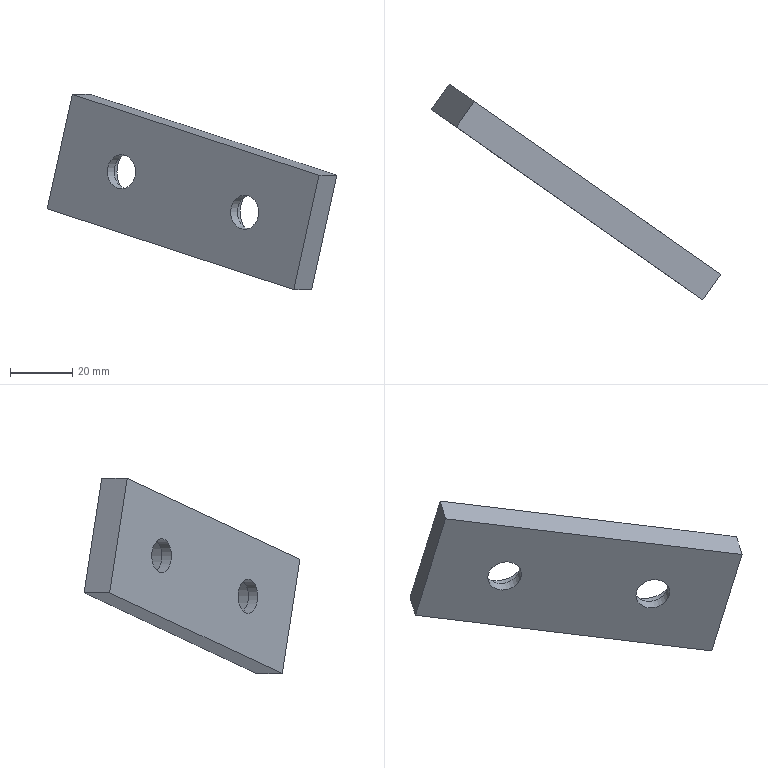Part | NX | features solid 2 | 1 solid | 12 faces | box 92.916 x 69.236 x 62.587 mm | volume 34266 mm3 | plane 8 | cylinder 4 | commonest cylinder face diameters 11 x2 17.5 x2
STEP:
#1=CARTESIAN_POINT('',(-114.685,856.129,30.673));
#2=VERTEX_POINT('',#1);
#3=CARTESIAN_POINT('',(-35.561,800.726,4.791));
#4=VERTEX_POINT('',#3);
#5=CARTESIAN_POINT('',(-109.761,852.681,29.063));
#6=DIRECTION('',(0.7912,-0.554,-0.2588));
#7=VECTOR('',#6,1000.);
#8=LINE('',#5,#7);
#9=EDGE_CURVE('',#2,#4,#8,.T.);
#10=ORIENTED_EDGE('',*,*,#9,.T.);
#11=CARTESIAN_POINT('',(-29.825,808.918,4.791));
#12=VERTEX_POINT('',#11);
#13=CARTESIAN_POINT('',(-29.825,808.918,4.791));
#14=DIRECTION('',(-0.5736,-0.8192,0.));
#15=VECTOR('',#14,1000.);
#16=LINE('',#13,#15);
#17=EDGE_CURVE('',#12,#4,#16,.T.);
#18=ORIENTED_EDGE('',*,*,#17,.F.);
#19=CARTESIAN_POINT('',(-108.949,864.321,30.673));
#20=VERTEX_POINT('',#19);
#21=CARTESIAN_POINT('',(-104.025,860.873,29.063));
#22=DIRECTION('',(0.7912,-0.554,-0.2588));
#23=VECTOR('',#22,1000.);
#24=LINE('',#21,#23);
#25=EDGE_CURVE('',#20,#12,#24,.T.);
#26=ORIENTED_EDGE('',*,*,#25,.F.);
#27=CARTESIAN_POINT('',(-108.949,864.321,30.673));
#28=DIRECTION('',(-0.5736,-0.8192,0.));
#29=VECTOR('',#28,1000.);
#30=LINE('',#27,#29);
#31=EDGE_CURVE('',#20,#2,#30,.T.);
#32=ORIENTED_EDGE('',*,*,#31,.T.);
#33=EDGE_LOOP('',(#10,#18,#26,#32));
#34=FACE_BOUND('',#33,.T.);
#35=CARTESIAN_POINT('',(-104.025,860.873,29.063));
#36=DIRECTION('',(0.212,-0.1485,0.9659));
#37=DIRECTION('',(-0.9676,-0.1706,0.1862));
#38=AXIS2_PLACEMENT_3D('',#35,#36,#37);
#39=PLANE('',#38);
#40=ADVANCED_FACE('',(#34),#39,.T.);
#41=CARTESIAN_POINT('',(-122.741,861.77,-6.032));
#42=VERTEX_POINT('',#41);
#43=CARTESIAN_POINT('',(-133.766,869.49,-56.26));
#44=DIRECTION('',(0.212,-0.1485,0.9659));
#45=VECTOR('',#44,1000.);
#46=LINE('',#43,#45);
#47=EDGE_CURVE('',#42,#2,#46,.T.);
#48=ORIENTED_EDGE('',*,*,#47,.T.);
#49=ORIENTED_EDGE('',*,*,#31,.F.);
#50=CARTESIAN_POINT('',(-117.005,869.962,-6.032));
#51=VERTEX_POINT('',#50);
#52=CARTESIAN_POINT('',(-128.03,877.681,-56.26));
#53=DIRECTION('',(0.212,-0.1485,0.9659));
#54=VECTOR('',#53,1000.);
#55=LINE('',#52,#54);
#56=EDGE_CURVE('',#51,#20,#55,.T.);
#57=ORIENTED_EDGE('',*,*,#56,.F.);
#58=CARTESIAN_POINT('',(-117.005,869.962,-6.032));
#59=DIRECTION('',(-0.5736,-0.8192,0.));
#60=VECTOR('',#59,1000.);
#61=LINE('',#58,#60);
#62=EDGE_CURVE('',#51,#42,#61,.T.);
#63=ORIENTED_EDGE('',*,*,#62,.T.);
#64=EDGE_LOOP('',(#48,#49,#57,#63));
#65=FACE_BOUND('',#64,.T.);
#66=CARTESIAN_POINT('',(-128.03,877.681,-56.26));
#67=DIRECTION('',(-0.7912,0.554,0.2588));
#68=DIRECTION('',(0.5736,0.8192,0.));
#69=AXIS2_PLACEMENT_3D('',#66,#67,#68);
#70=PLANE('',#69);
#71=ADVANCED_FACE('',(#65),#70,.T.);
#72=CARTESIAN_POINT('',(-43.617,806.367,-31.914));
#73=VERTEX_POINT('',#72);
#74=CARTESIAN_POINT('',(-117.817,858.323,-7.643));
#75=DIRECTION('',(0.7912,-0.554,-0.2588));
#76=VECTOR('',#75,1000.);
#77=LINE('',#74,#76);
#78=EDGE_CURVE('',#42,#73,#77,.T.);
#79=ORIENTED_EDGE('',*,*,#78,.F.);
#80=ORIENTED_EDGE('',*,*,#62,.F.);
#81=CARTESIAN_POINT('',(-37.881,814.559,-31.914));
#82=VERTEX_POINT('',#81);
#83=CARTESIAN_POINT('',(-112.081,866.514,-7.643));
#84=DIRECTION('',(0.7912,-0.554,-0.2588));
#85=VECTOR('',#84,1000.);
#86=LINE('',#83,#85);
#87=EDGE_CURVE('',#51,#82,#86,.T.);
#88=ORIENTED_EDGE('',*,*,#87,.T.);
#89=CARTESIAN_POINT('',(-37.881,814.559,-31.914));
#90=DIRECTION('',(-0.5736,-0.8192,0.));
#91=VECTOR('',#90,1000.);
#92=LINE('',#89,#91);
#93=EDGE_CURVE('',#82,#73,#92,.T.);
#94=ORIENTED_EDGE('',*,*,#93,.T.);
#95=EDGE_LOOP('',(#79,#80,#88,#94));
#96=FACE_BOUND('',#95,.T.);
#97=CARTESIAN_POINT('',(-112.081,866.514,-7.643));
#98=DIRECTION('',(0.212,-0.1485,0.9659));
#99=DIRECTION('',(-0.9676,-0.1706,0.1862));
#100=AXIS2_PLACEMENT_3D('',#97,#98,#99);
#101=PLANE('',#100);
#102=ADVANCED_FACE('',(#96),#101,.F.);
#103=CARTESIAN_POINT('',(-54.642,814.087,-82.142));
#104=DIRECTION('',(0.212,-0.1485,0.9659));
#105=VECTOR('',#104,1000.);
#106=LINE('',#103,#105);
#107=EDGE_CURVE('',#73,#4,#106,.T.);
#108=ORIENTED_EDGE('',*,*,#107,.F.);
#109=ORIENTED_EDGE('',*,*,#93,.F.);
#110=CARTESIAN_POINT('',(-48.906,822.278,-82.142));
#111=DIRECTION('',(0.212,-0.1485,0.9659));
#112=VECTOR('',#111,1000.);
#113=LINE('',#110,#112);
#114=EDGE_CURVE('',#82,#12,#113,.T.);
#115=ORIENTED_EDGE('',*,*,#114,.T.);
#116=ORIENTED_EDGE('',*,*,#17,.T.);
#117=EDGE_LOOP('',(#108,#109,#115,#116));
#118=FACE_BOUND('',#117,.T.);
#119=CARTESIAN_POINT('',(-48.906,822.278,-82.142));
#120=DIRECTION('',(-0.7912,0.554,0.2588));
#121=DIRECTION('',(0.5736,0.8192,0.));
#122=AXIS2_PLACEMENT_3D('',#119,#120,#121);
#123=PLANE('',#122);
#124=ADVANCED_FACE('',(#118),#123,.F.);
#125=CARTESIAN_POINT('',(-86.028,848.272,5.85));
#126=VERTEX_POINT('',#125);
#127=CARTESIAN_POINT('',(-93.196,853.291,5.85));
#128=DIRECTION('',(-0.5736,-0.8192,0.));
#129=DIRECTION('',(0.8192,-0.5736,0.));
#130=AXIS2_PLACEMENT_3D('',#127,#128,#129);
#131=CIRCLE('',#130,8.75);
#132=EDGE_CURVE('',#126,#126,#131,.T.);
#133=ORIENTED_EDGE('',*,*,#132,.T.);
#134=EDGE_LOOP('',(#133));
#135=FACE_BOUND('',#134,.T.);
#136=CARTESIAN_POINT('',(-46.466,820.57,-7.091));
#137=VERTEX_POINT('',#136);
#138=CARTESIAN_POINT('',(-53.634,825.589,-7.091));
#139=DIRECTION('',(-0.5736,-0.8192,0.));
#140=DIRECTION('',(0.8192,-0.5736,0.));
#141=AXIS2_PLACEMENT_3D('',#138,#139,#140);
#142=CIRCLE('',#141,8.75);
#143=EDGE_CURVE('',#137,#137,#142,.T.);
#144=ORIENTED_EDGE('',*,*,#143,.T.);
#145=EDGE_LOOP('',(#144));
#146=FACE_BOUND('',#145,.T.);
#147=ORIENTED_EDGE('',*,*,#25,.T.);
#148=ORIENTED_EDGE('',*,*,#114,.F.);
#149=ORIENTED_EDGE('',*,*,#87,.F.);
#150=ORIENTED_EDGE('',*,*,#56,.T.);
#151=EDGE_LOOP('',(#147,#148,#149,#150));
#152=FACE_BOUND('',#151,.T.);
#153=CARTESIAN_POINT('',(-123.106,874.234,-57.871));
#154=DIRECTION('',(0.5736,0.8192,0.));
#155=DIRECTION('',(0.8192,-0.5736,0.));
#156=AXIS2_PLACEMENT_3D('',#153,#154,#155);
#157=PLANE('',#156);
#158=ADVANCED_FACE('',(#135,#146,#152),#157,.T.);
#159=CARTESIAN_POINT('',(-103.437,848.254,5.85));
#160=VERTEX_POINT('',#159);
#161=CARTESIAN_POINT('',(-98.932,845.099,5.85));
#162=DIRECTION('',(0.5736,0.8192,0.));
#163=DIRECTION('',(-0.8192,0.5736,0.));
#164=AXIS2_PLACEMENT_3D('',#161,#162,#163);
#165=CIRCLE('',#164,5.5);
#166=EDGE_CURVE('',#160,#160,#165,.T.);
#167=ORIENTED_EDGE('',*,*,#166,.T.);
#168=EDGE_LOOP('',(#167));
#169=FACE_BOUND('',#168,.T.);
#170=CARTESIAN_POINT('',(-63.875,820.552,-7.091));
#171=VERTEX_POINT('',#170);
#172=CARTESIAN_POINT('',(-59.37,817.397,-7.091));
#173=DIRECTION('',(0.5736,0.8192,0.));
#174=DIRECTION('',(-0.8192,0.5736,0.));
#175=AXIS2_PLACEMENT_3D('',#172,#173,#174);
#176=CIRCLE('',#175,5.5);
#177=EDGE_CURVE('',#171,#171,#176,.T.);
#178=ORIENTED_EDGE('',*,*,#177,.T.);
#179=EDGE_LOOP('',(#178));
#180=FACE_BOUND('',#179,.T.);
#181=ORIENTED_EDGE('',*,*,#9,.F.);
#182=ORIENTED_EDGE('',*,*,#47,.F.);
#183=ORIENTED_EDGE('',*,*,#78,.T.);
#184=ORIENTED_EDGE('',*,*,#107,.T.);
#185=EDGE_LOOP('',(#181,#182,#183,#184));
#186=FACE_BOUND('',#185,.T.);
#187=CARTESIAN_POINT('',(-128.842,866.042,-57.871));
#188=DIRECTION('',(0.5736,0.8192,0.));
#189=DIRECTION('',(0.8192,-0.5736,0.));
#190=AXIS2_PLACEMENT_3D('',#187,#188,#189);
#191=PLANE('',#190);
#192=ADVANCED_FACE('',(#169,#180,#186),#191,.F.);
#193=CARTESIAN_POINT('',(-52.742,817.274,-7.091));
#194=VERTEX_POINT('',#193);
#195=CARTESIAN_POINT('',(-57.248,820.428,-7.091));
#196=DIRECTION('',(-0.5736,-0.8192,0.));
#197=DIRECTION('',(0.8192,-0.5736,0.));
#198=AXIS2_PLACEMENT_3D('',#195,#196,#197);
#199=CIRCLE('',#198,5.5);
#200=EDGE_CURVE('',#194,#194,#199,.T.);
#201=ORIENTED_EDGE('',*,*,#200,.F.);
#202=EDGE_LOOP('',(#201));
#203=FACE_BOUND('',#202,.T.);
#204=ORIENTED_EDGE('',*,*,#177,.F.);
#205=EDGE_LOOP('',(#204));
#206=FACE_BOUND('',#205,.T.);
#207=CARTESIAN_POINT('',(-82.313,784.631,-7.091));
#208=DIRECTION('',(-0.5736,-0.8192,0.));
#209=DIRECTION('',(0.8192,-0.5736,0.));
#210=AXIS2_PLACEMENT_3D('',#207,#208,#209);
#211=CYLINDRICAL_SURFACE('',#210,5.5);
#212=ADVANCED_FACE('',(#203,#206),#211,.F.);
#213=ORIENTED_EDGE('',*,*,#200,.T.);
#214=EDGE_LOOP('',(#213));
#215=FACE_BOUND('',#214,.T.);
#216=CARTESIAN_POINT('',(-50.08,815.409,-7.091));
#217=VERTEX_POINT('',#216);
#218=CARTESIAN_POINT('',(-57.248,820.428,-7.091));
#219=DIRECTION('',(-0.5736,-0.8192,0.));
#220=DIRECTION('',(0.8192,-0.5736,0.));
#221=AXIS2_PLACEMENT_3D('',#218,#219,#220);
#222=CIRCLE('',#221,8.75);
#223=EDGE_CURVE('',#217,#217,#222,.T.);
#224=ORIENTED_EDGE('',*,*,#223,.F.);
#225=EDGE_LOOP('',(#224));
#226=FACE_BOUND('',#225,.T.);
#227=CARTESIAN_POINT('',(-56.187,819.686,-2.261));
#228=DIRECTION('',(-0.5736,-0.8192,0.));
#229=DIRECTION('',(0.8192,-0.5736,0.));
#230=AXIS2_PLACEMENT_3D('',#227,#228,#229);
#231=PLANE('',#230);
#232=ADVANCED_FACE('',(#215,#226),#231,.F.);
#233=ORIENTED_EDGE('',*,*,#223,.T.);
#234=EDGE_LOOP('',(#233));
#235=FACE_BOUND('',#234,.T.);
#236=ORIENTED_EDGE('',*,*,#143,.F.);
#237=EDGE_LOOP('',(#236));
#238=FACE_BOUND('',#237,.T.);
#239=CARTESIAN_POINT('',(-53.634,825.589,-7.091));
#240=DIRECTION('',(-0.5736,-0.8192,0.));
#241=DIRECTION('',(0.8192,-0.5736,0.));
#242=AXIS2_PLACEMENT_3D('',#239,#240,#241);
#243=CYLINDRICAL_SURFACE('',#242,8.75);
#244=ADVANCED_FACE('',(#235,#238),#243,.F.);
#245=CARTESIAN_POINT('',(-92.304,844.975,5.85));
#246=VERTEX_POINT('',#245);
#247=CARTESIAN_POINT('',(-96.81,848.13,5.85));
#248=DIRECTION('',(-0.5736,-0.8192,0.));
#249=DIRECTION('',(0.8192,-0.5736,0.));
#250=AXIS2_PLACEMENT_3D('',#247,#248,#249);
#251=CIRCLE('',#250,5.5);
#252=EDGE_CURVE('',#246,#246,#251,.T.);
#253=ORIENTED_EDGE('',*,*,#252,.F.);
#254=EDGE_LOOP('',(#253));
#255=FACE_BOUND('',#254,.T.);
#256=ORIENTED_EDGE('',*,*,#166,.F.);
#257=EDGE_LOOP('',(#256));
#258=FACE_BOUND('',#257,.T.);
#259=CARTESIAN_POINT('',(-121.875,812.333,5.85));
#260=DIRECTION('',(-0.5736,-0.8192,0.));
#261=DIRECTION('',(0.8192,-0.5736,0.));
#262=AXIS2_PLACEMENT_3D('',#259,#260,#261);
#263=CYLINDRICAL_SURFACE('',#262,5.5);
#264=ADVANCED_FACE('',(#255,#258),#263,.F.);
#265=ORIENTED_EDGE('',*,*,#252,.T.);
#266=EDGE_LOOP('',(#265));
#267=FACE_BOUND('',#266,.T.);
#268=CARTESIAN_POINT('',(-89.642,843.111,5.85));
#269=VERTEX_POINT('',#268);
#270=CARTESIAN_POINT('',(-96.81,848.13,5.85));
#271=DIRECTION('',(-0.5736,-0.8192,0.));
#272=DIRECTION('',(0.8192,-0.5736,0.));
#273=AXIS2_PLACEMENT_3D('',#270,#271,#272);
#274=CIRCLE('',#273,8.75);
#275=EDGE_CURVE('',#269,#269,#274,.T.);
#276=ORIENTED_EDGE('',*,*,#275,.F.);
#277=EDGE_LOOP('',(#276));
#278=FACE_BOUND('',#277,.T.);
#279=CARTESIAN_POINT('',(-95.749,847.388,10.68));
#280=DIRECTION('',(-0.5736,-0.8192,0.));
#281=DIRECTION('',(0.8192,-0.5736,0.));
#282=AXIS2_PLACEMENT_3D('',#279,#280,#281);
#283=PLANE('',#282);
#284=ADVANCED_FACE('',(#267,#278),#283,.F.);
#285=ORIENTED_EDGE('',*,*,#275,.T.);
#286=EDGE_LOOP('',(#285));
#287=FACE_BOUND('',#286,.T.);
#288=ORIENTED_EDGE('',*,*,#132,.F.);
#289=EDGE_LOOP('',(#288));
#290=FACE_BOUND('',#289,.T.);
#291=CARTESIAN_POINT('',(-93.196,853.291,5.85));
#292=DIRECTION('',(-0.5736,-0.8192,0.));
#293=DIRECTION('',(0.8192,-0.5736,0.));
#294=AXIS2_PLACEMENT_3D('',#291,#292,#293);
#295=CYLINDRICAL_SURFACE('',#294,8.75);
#296=ADVANCED_FACE('',(#287,#290),#295,.F.);
#297=CLOSED_SHELL('',(#40,#71,#102,#124,#158,#192,#212,#232,#244,#264,#284,#296));
#298=MANIFOLD_SOLID_BREP('',#297);
#299=(LENGTH_UNIT()NAMED_UNIT(*)SI_UNIT(.MILLI.,.METRE.));
#300=UNCERTAINTY_MEASURE_WITH_UNIT(LENGTH_MEASURE(0.00001),#299,'','');
#301=(NAMED_UNIT(*)PLANE_ANGLE_UNIT()SI_UNIT($,.RADIAN.));
#302=(NAMED_UNIT(*)SI_UNIT($,.STERADIAN.)SOLID_ANGLE_UNIT());
#303=(GEOMETRIC_REPRESENTATION_CONTEXT(3)GLOBAL_UNCERTAINTY_ASSIGNED_CONTEXT((#300))GLOBAL_UNIT_ASSIGNED_CONTEXT((#299,#301,#302))REPRESENTATION_CONTEXT('',''));
#304=ADVANCED_BREP_SHAPE_REPRESENTATION('',(#298),#303);